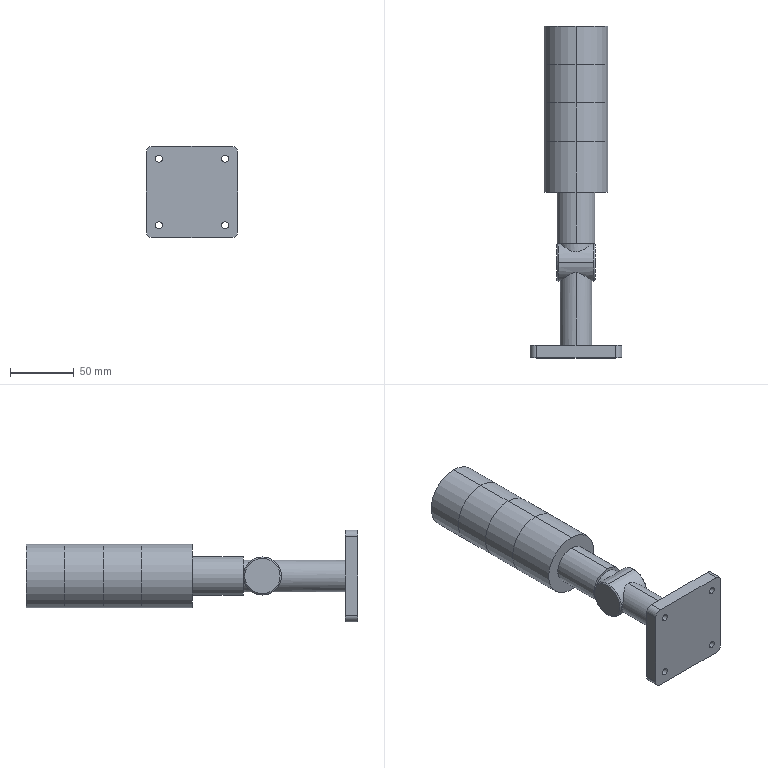Part | SolidWorks | features BaseBody 4 | 4 solids | 50 faces | box 72 x 260.521 x 72 mm | volume 382291 mm3 | cylinder 29 | plane 17 | cone 4 | commonest cylinder face diameters 5.5 x8 50 x8 25 x5 10 x4 29.842 x2 30 x2